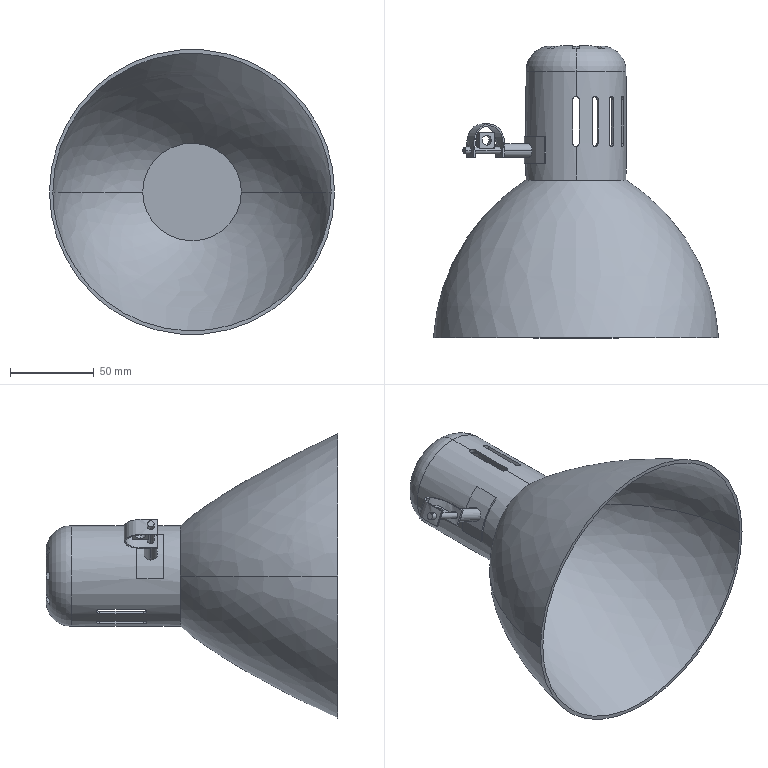Part | SolidWorks | features CompositeCurve 4 | 4 solids | 128 faces | box 170 x 174.745 x 170 mm | volume 120724 mm3 | plane 77 | cylinder 39 | spline 8 | torus 4 | commonest cylinder face diameters 4 x28 6 x2 8 x2 56 x2 60 x2 0.56 x1